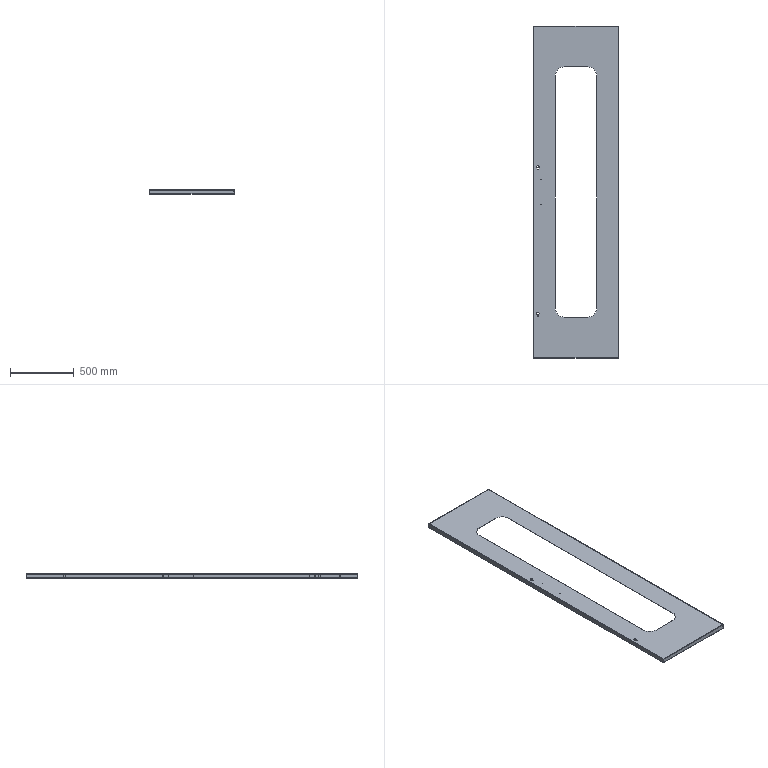Part | SolidWorks | features Cut 8, EdgeFlange 2, ICE 2, FlatPattern 1, SMBaseFlange 1, SheetMetal 1 | 1 solid | 116 faces | box 666 x 2594 x 35 mm | volume 2126222 mm3 | cylinder 54 | plane 46 | spline 16 | commonest cylinder face diameters 5.5 x12 3 x8 6 x8 19 x6 4 x4 8 x4